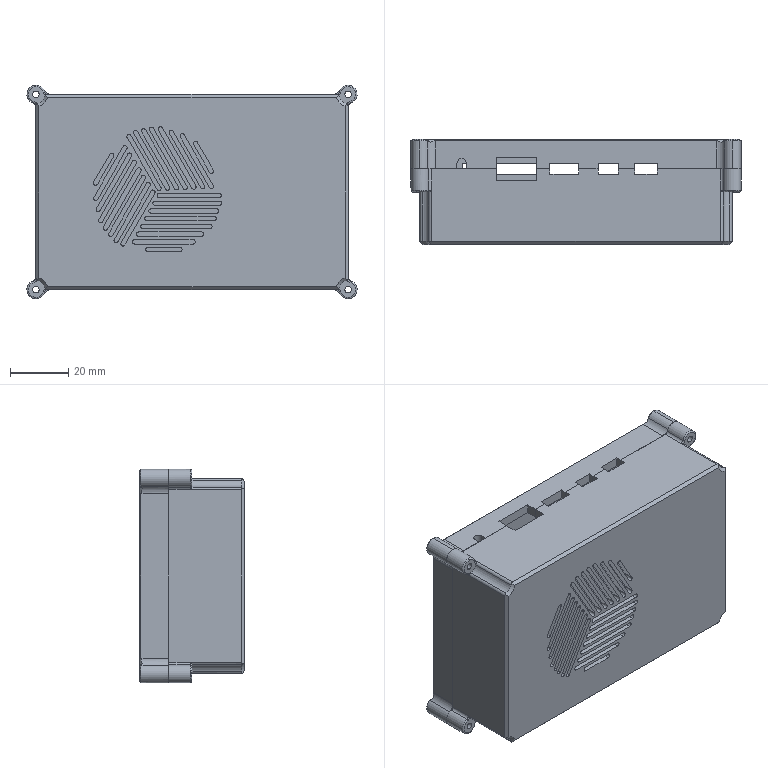Part | SolidWorks | 2 solids | 481 faces | box 113.2 x 36 x 73.2 mm | volume 73752 mm3 | cylinder 224 | plane 203 | spline 38 | cone 16 | commonest cylinder face diameters 2 x88 1.5 x64 2.2 x16 6.2 x16 6 x12 3.5 x9